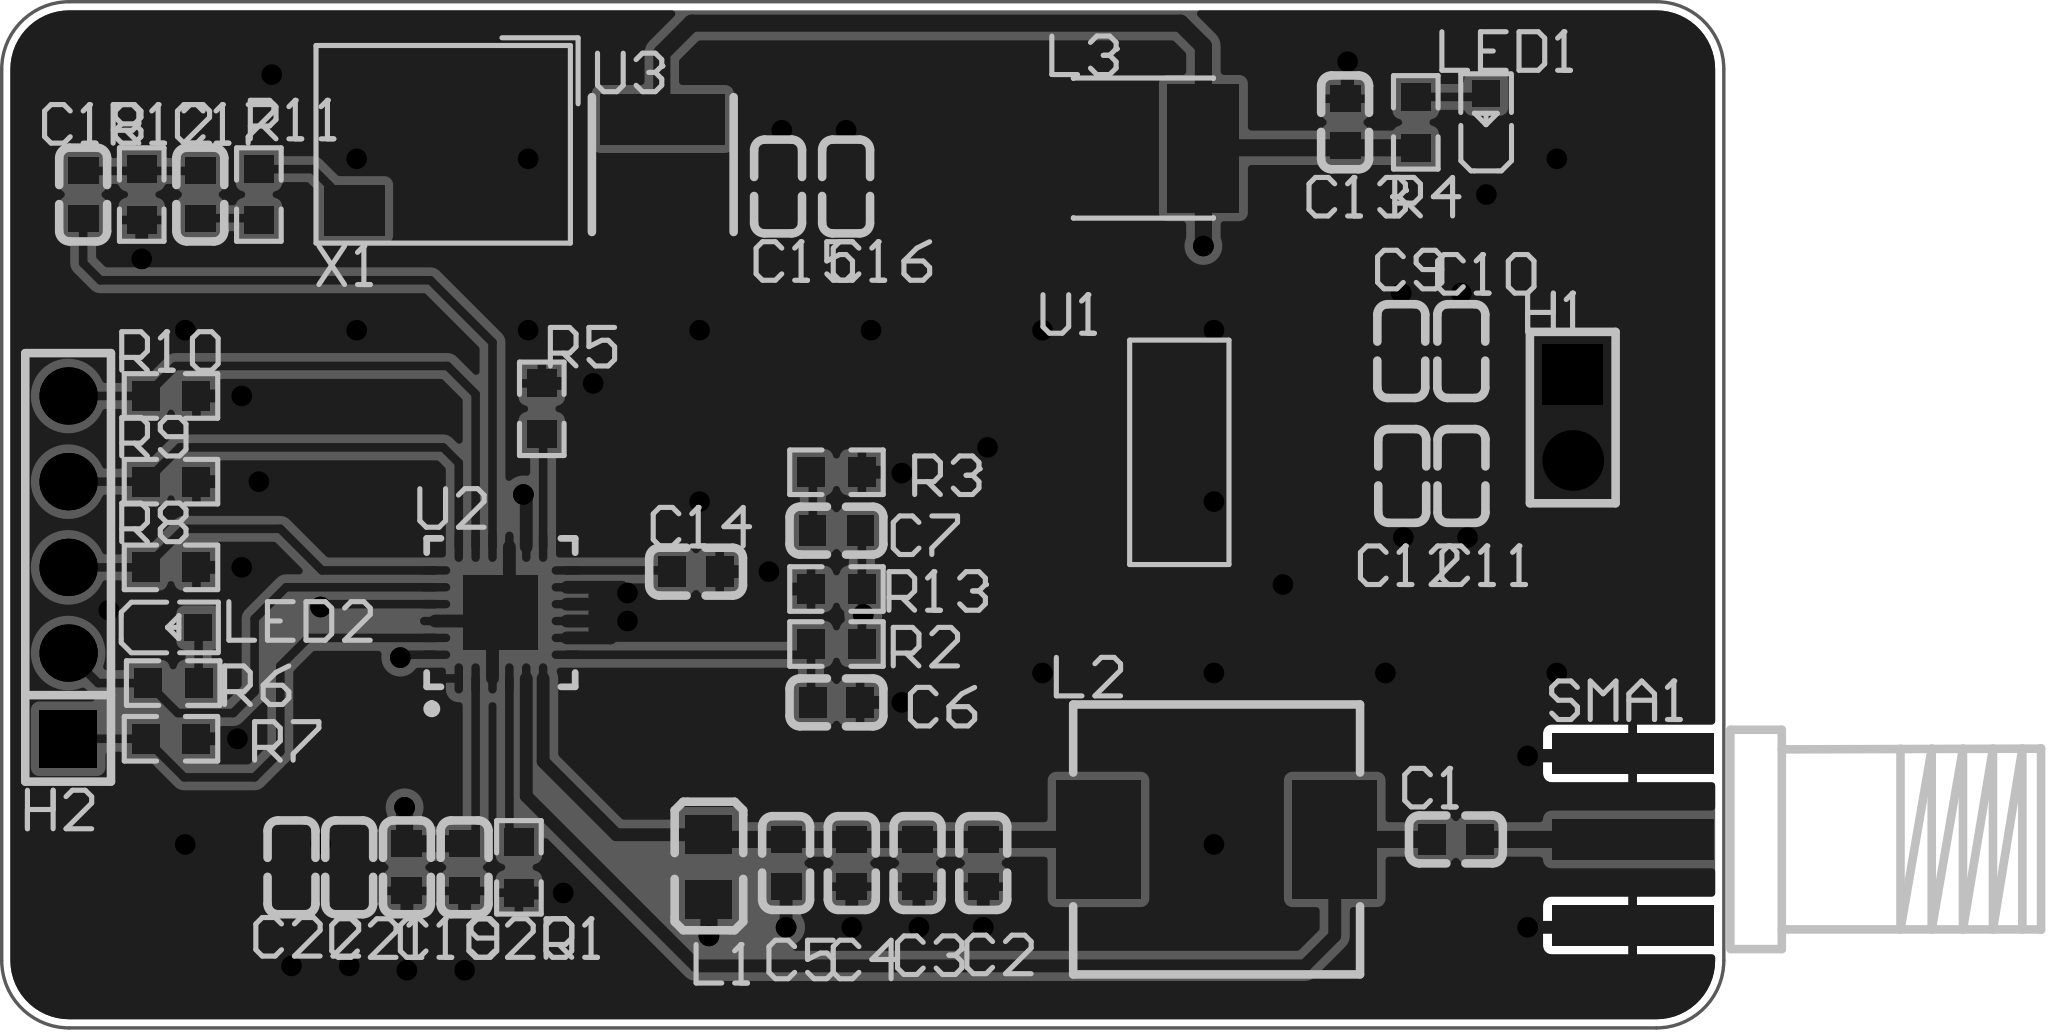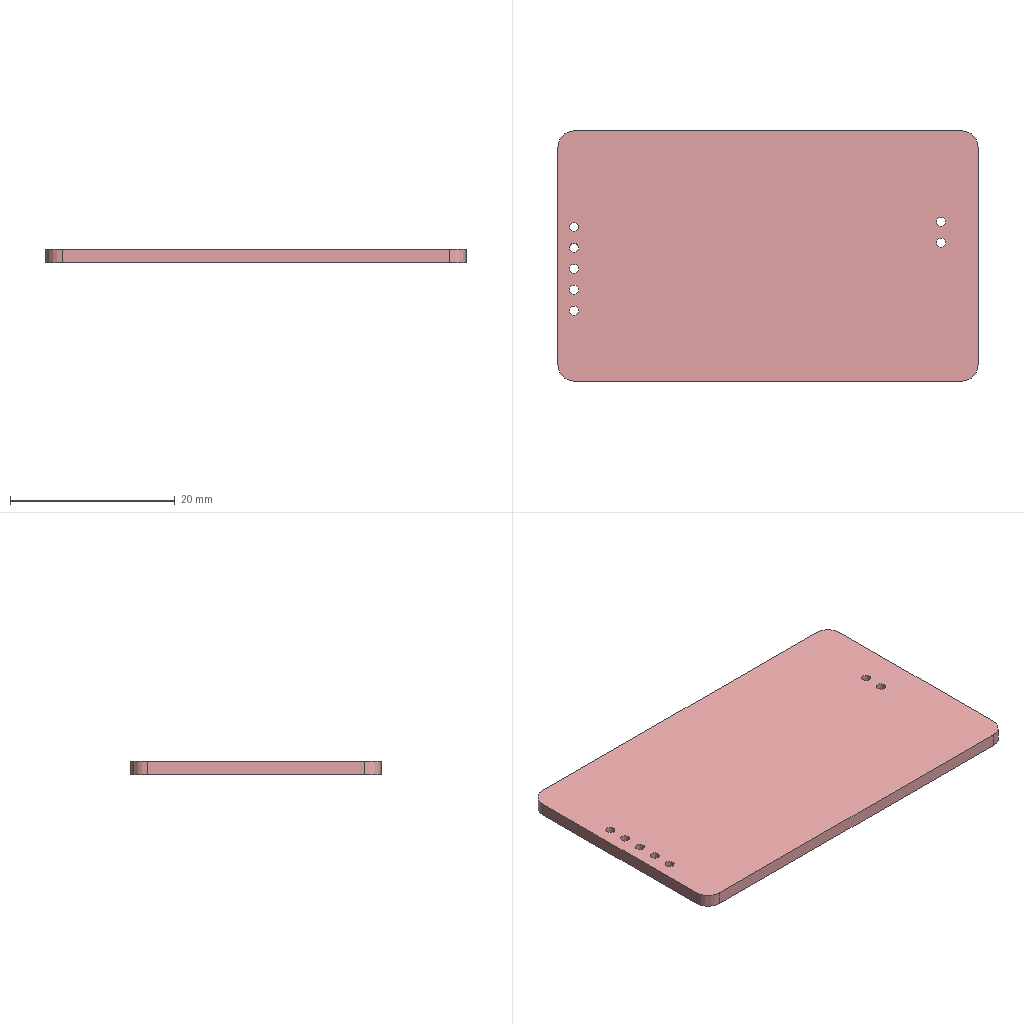Circuit board layout | Altium Designer | box 51 x 30.4 x 1.6 mm
Layer stack:
# Altium Designer layer stack of  (unit mm; dielectric type: 0 none, 1 core, 2 prepreg, 3 surface material)
index,name,kind,layer,copper_thickness_mm,dielectric_type,dielectric_thickness_mm,dielectric_material,dielectric_constant
0,Top Paste Mask Layer,other,,,,,,
1,Top Silkscreen Layer,other,,,,,,
2,Top Solder Mask Layer,dielectric,,,3,0.01,,3.3
3,Top Layer,copper,Top Layer,0.035,,,,
4,Dielectric1,dielectric,,,3,1.51,FR4,4.5
5,Bottom Layer,copper,Bottom Layer,0.035,,,,
6,Bottom Solder Mask Layer,dielectric,,,3,0.01,,3.3
7,Bottom Silkscreen Layer,other,,,,,,
8,Bottom Paste Mask Layer,other,,,,,,
# drill layer pairs: low layer,high layer
drill_pair,Top Layer,Bottom Layer
Part placement:
Designator,Comment,Layer,Footprint,Center-X(mm),Center-Y(mm),Rotation
C1,10pF,TopLayer,C0603,120.811,84.012,0
C2,10pF,TopLayer,C0603,106.807,83.312,90
C3,10pF,TopLayer,C0603,104.86,83.312,90
C4,10pF,TopLayer,C0603,102.912,83.312,90
C5,10nF,TopLayer,C0603,100.965,83.312,90
C6,33pF,TopLayer,C0603,102.457,88.073,180
C7,150pF,TopLayer,C0603,102.457,93.164,0
C9,0.1uF,TopLayer,C0603,119.193,98.484,270
C10,47uF,TopLayer,C0603,120.971,98.484,270
C11,0.1uF,TopLayer,C0603,120.977,94.784,90
C12,10uF,TopLayer,C0603,119.221,94.784,90
C13,10uF,TopLayer,C0603,117.528,105.263,270
C14,1nF,TopLayer,C0603,98.298,91.948,180
C15,100pF,TopLayer,C0603,100.727,103.363,270
C16,0.1uF,TopLayer,C0603,102.743,103.363,270
C17,1nF,TopLayer,C0603,83.608,103.124,90
C18,1nF,TopLayer,C0603,80.137,103.124,270
C19,100pF,TopLayer,C0603,89.73,83.185,90
C20,0.1uF,TopLayer,C0603,91.44,83.185,90
C21,100pF,TopLayer,C0603,88.021,83.185,90
C22,0.1uF,TopLayer,C0603,86.311,83.185,90
H1,,TopLayer,HDR-TH_2P-P2.54-V-M-1,124.273,96.514,270
H2,,TopLayer,HDR-TH_5P-P2.54-V-M,79.692,92.075,90
L1,100nH,TopLayer,L0805,98.679,83.185,270
L2,15uH,TopLayer,IND-SMD_L8.5-W8.0-LS9.5_ZEYH0850-15UH,113.721,84.012,0
L3,100uH,TopLayer,IND-SMD_L4.0-W4.0_SWPA4018S,111.552,104.501,180
LED1,,TopLayer,LED_0603,121.712,105.313,90
LED2,,TopLayer,LED_0603,82.753,90.289,0
R1,51R,TopLayer,R0603,93.049,83.185,90
R2,0KR,TopLayer,R0603,102.457,89.803,180
R3,13KR,TopLayer,R0603,102.457,94.894,0
R4,51R,TopLayer,R0603,119.623,105.263,270
R5,4.7KR,TopLayer,R0603,93.726,96.774,270
R6,1KR,TopLayer,R0603,82.804,88.646,180
R7,10KR,TopLayer,R0603,82.74,86.995,0
R8,10KR,TopLayer,R0603,82.74,92.075,0
R9,10KR,TopLayer,R0603,82.74,94.615,0
R10,10KR,TopLayer,R0603,82.74,97.155,0
R11,0R,TopLayer,R0603,85.344,103.124,90
R12,51R,TopLayer,R0603,81.873,103.124,270
SMA1,SMA,TopLayer,SMA-SMD_BWSMA-KE-P001,126.049,84.012,0
U1,AMS1117-3.3,TopLayer,SOT-223-3_L6.5-W3.4-P2.30-LS7.0-BR,112.716,95.484,0
U2,ADF4360-0BCPZ,TopLayer,LFCSP-24_L4.0-W4.0-P0.50-BL-EP2.3,92.516,90.735,0
U3,10uH,TopLayer,IND-SMD_L4.0-W4.0_LVF404015,97.311,104.013,270
X1,16MHz,TopLayer,OSC-SMD_4P-L7.0-W5.0-BL,90.805,104.613,180
R13,NC,TopLayer,R0603,102.457,91.433,180
Pad and via stacks:
# Altium Designer via and pad stacks of  (unit mm). Each distinct definition once, with the count of objects using it.
# via: kind,start_layer,end_layer,hole_mm,diameter_mm,mode(0 simple;1 top-mid-bottom;2 full stack),diameter_per_layer,count,example_net
# pad: kind,layer,hole_mm,hole_type(0 round;1 square;2 slot),plating,top_size,top_shape(1 round;2 rect;3 octagon;9 rounded rect),mid_size,bottom_size,mode,footprint,size_per_layer,count,example
pad,Top Layer,0,0,plated,0.8x0.9,2,0.8x0.9,0.8x0.9,0,C0603,,42,C1.2
pad,Top Layer,0,0,plated,1.133x1.377,2,1.133x1.377,1.133x1.377,0,L0805,,2,L1.1
pad,Top Layer,0,0,plated,2.5x3.5,2,2.5x3.5,2.5x3.5,0,IND-SMD_L8.5-W8.0-LS9.5_ZEYH0850-15UH,,2,L2.1
pad,Top Layer,0,0,plated,2.124x3.82,2,2.124x3.82,2.124x3.82,0,IND-SMD_L4.0-W4.0_SWPA4018S,,2,L3.1
pad,Top Layer,0,0,plated,0.8001x0.8001,2,0.8001x0.8001,0.8001x0.8001,0,LED_0603,,4,LED1.1
pad,Top Layer,0,0,plated,0.8065x0.864,2,0.8065x0.864,0.8065x0.864,0,R0603,,26,R1.2
pad,Top Layer,0,0,plated,4.8x1.2,2,4.8x1.2,4.8x1.2,0,SMA-SMD_BWSMA-KE-P001,,3,SMA1.1
pad,Top Layer,0,0,plated,2.5x1.1,2,2.5x1.1,2.5x1.1,0,SOT-223-3_L6.5-W3.4-P2.30-LS7.0-BR,,3,U1.1
pad,Top Layer,0,0,plated,2.34x3.6,2,2.34x3.6,2.34x3.6,0,SOT-223-3_L6.5-W3.4-P2.30-LS7.0-BR,,1,U1.4
pad,Top Layer,0,0,plated,0.9x0.25,1,0.9x0.25,0.9x0.25,0,LFCSP-24_L4.0-W4.0-P0.50-BL-EP2.3,,12,U2.24
pad,Top Layer,0,0,plated,0.25x0.9,1,0.25x0.9,0.25x0.9,0,LFCSP-24_L4.0-W4.0-P0.50-BL-EP2.3,,12,U2.18
pad,Top Layer,0,0,plated,2.2x2.2,2,2.2x2.2,2.2x2.2,0,LFCSP-24_L4.0-W4.0-P0.50-BL-EP2.3,,1,U2.25
pad,Top Layer,0,0,plated,3.7x1.5,2,3.7x1.5,3.7x1.5,0,IND-SMD_L4.0-W4.0_LVF404015,,2,U3.1
pad,Top Layer,0,0,plated,1.8x1.5,2,1.8x1.5,1.8x1.5,0,OSC-SMD_4P-L7.0-W5.0-BL,,4,X1.1
pad,Multi-Layer,1.1,0,plated,1.8x1.8,1,1.8x1.8,1.8x1.8,0,HDR-TH_2P-P2.54-V-M-1,,1,H1.2
pad,Multi-Layer,1.1,0,plated,1.8x1.8,2,1.8x1.8,1.8x1.8,0,HDR-TH_2P-P2.54-V-M-1,,1,H1.1
pad,Multi-Layer,1.1,0,plated,1.7x1.7,2,1.7x1.7,1.7x1.7,0,HDR-TH_5P-P2.54-V-M,,1,H2.1
pad,Multi-Layer,1.1,0,plated,1.7x1.7,1,1.7x1.7,1.7x1.7,0,HDR-TH_5P-P2.54-V-M,,4,H2.2
pad,Bottom Layer,0,0,plated,4.8x1.2,2,4.8x1.2,4.8x1.2,0,SMA-SMD_BWSMA-KE-P001,,2,SMA1.3
via,Top Layer,Bottom Layer,0.3048,0.61,0,,66,DVDD
Copper pours:
name,layer,net,type(0 solid;1 hatched;2 none)
Top Layer-GND,Top Layer,GND,0
Bottom Layer-GND,Bottom Layer,GND,0